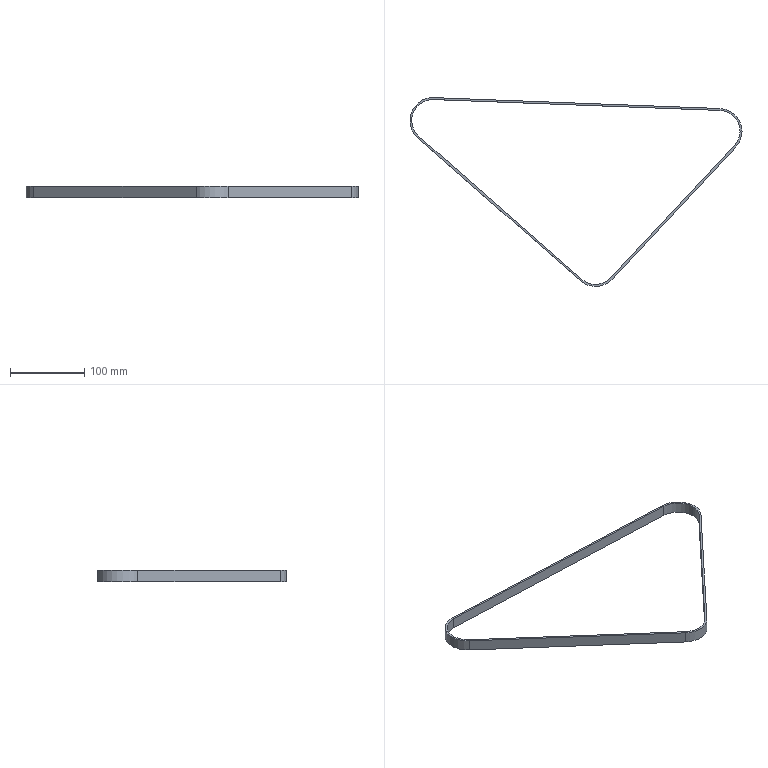Part | STEP file | Belt 2-5^ tube-changer assembly SGN-2 | 1 solid | 16 faces | box 446.051 x 253.563 x 15 mm | volume 43377 mm3 | cylinder 8 | plane 8 | commonest cylinder face diameters 56.34 x4 61.58 x4
STEP:
#1=CARTESIAN_POINT('',(0.,0.,0.));
#2=DIRECTION('',(0.,0.,1.));
#3=DIRECTION('',(1.,0.,0.));
#4=AXIS2_PLACEMENT_3D('',#1,#2,#3);
#5=CARTESIAN_POINT('',(-24.996,40.281,-15.));
#6=VERTEX_POINT('',#5);
#7=CARTESIAN_POINT('',(-24.996,40.281,0.));
#8=VERTEX_POINT('',#7);
#9=CARTESIAN_POINT('',(-24.996,40.281,-15.));
#10=DIRECTION('',(0.,0.,1.));
#11=VECTOR('',#10,1.);
#12=LINE('',#9,#11);
#13=CARTESIAN_POINT('',(-26.065,12.131,-15.));
#14=DIRECTION('',(0.,0.,1.));
#15=DIRECTION('',(1.,0.,0.));
#16=AXIS2_PLACEMENT_3D('',#13,#14,#15);
#17=CYLINDRICAL_SURFACE('',#16,28.17);
#18=CARTESIAN_POINT('',(1.533,0.));
#19=DIRECTION('',(0.,1.));
#20=VECTOR('',#19,1.);
#21=LINE('',#18,#20);
#22=(GEOMETRIC_REPRESENTATION_CONTEXT(2)PARAMETRIC_REPRESENTATION_CONTEXT()REPRESENTATION_CONTEXT('',''));
#23=DEFINITIONAL_REPRESENTATION('',(#21),#22);
#24=PCURVE('',#17,#23);
#25=CARTESIAN_POINT('',(-24.996,40.281,-15.));
#26=DIRECTION('',(0.03795,0.9993,0.));
#27=DIRECTION('',(-0.9993,0.03795,0.));
#28=AXIS2_PLACEMENT_3D('',#25,#26,#27);
#29=PLANE('',#28);
#30=CARTESIAN_POINT('',(0.,0.));
#31=DIRECTION('',(0.,1.));
#32=VECTOR('',#31,1.);
#33=LINE('',#30,#32);
#34=(GEOMETRIC_REPRESENTATION_CONTEXT(2)PARAMETRIC_REPRESENTATION_CONTEXT()REPRESENTATION_CONTEXT('',''));
#35=DEFINITIONAL_REPRESENTATION('',(#33),#34);
#36=PCURVE('',#29,#35);
#37=SURFACE_CURVE('',#12,(#24,#36),.PCURVE_S1.);
#38=EDGE_CURVE('',#6,#8,#37,.T.);
#39=ORIENTED_EDGE('',*,*,#38,.T.);
#40=CARTESIAN_POINT('',(2.105,12.131,0.));
#41=VERTEX_POINT('',#40);
#42=CARTESIAN_POINT('',(-26.065,12.131,0.));
#43=DIRECTION('',(0.,0.,1.));
#44=DIRECTION('',(1.,0.,0.));
#45=AXIS2_PLACEMENT_3D('',#42,#43,#44);
#46=CIRCLE('',#45,28.17);
#47=CARTESIAN_POINT('',(0.,15.));
#48=DIRECTION('',(1.,0.));
#49=VECTOR('',#48,1.);
#50=LINE('',#47,#49);
#51=(GEOMETRIC_REPRESENTATION_CONTEXT(2)PARAMETRIC_REPRESENTATION_CONTEXT()REPRESENTATION_CONTEXT('',''));
#52=DEFINITIONAL_REPRESENTATION('',(#50),#51);
#53=PCURVE('',#17,#52);
#54=CARTESIAN_POINT('',(-26.065,12.131,0.));
#55=DIRECTION('',(0.,0.,1.));
#56=DIRECTION('',(1.,0.,0.));
#57=AXIS2_PLACEMENT_3D('',#54,#55,#56);
#58=PLANE('',#57);
#59=CARTESIAN_POINT('',(0.,0.));
#60=DIRECTION('',(1.,0.));
#61=AXIS2_PLACEMENT_2D('',#59,#60);
#62=CIRCLE('',#61,28.17);
#63=(GEOMETRIC_REPRESENTATION_CONTEXT(2)PARAMETRIC_REPRESENTATION_CONTEXT()REPRESENTATION_CONTEXT('',''));
#64=DEFINITIONAL_REPRESENTATION('',(#62),#63);
#65=PCURVE('',#58,#64);
#66=SURFACE_CURVE('',#46,(#53,#65),.PCURVE_S1.);
#67=EDGE_CURVE('',#41,#8,#66,.T.);
#68=ORIENTED_EDGE('',*,*,#67,.F.);
#69=CARTESIAN_POINT('',(2.105,12.131,-15.));
#70=VERTEX_POINT('',#69);
#71=CARTESIAN_POINT('',(2.105,12.131,-15.));
#72=DIRECTION('',(0.,0.,1.));
#73=VECTOR('',#72,1.);
#74=LINE('',#71,#73);
#75=CARTESIAN_POINT('',(0.,0.));
#76=DIRECTION('',(0.,1.));
#77=VECTOR('',#76,1.);
#78=LINE('',#75,#77);
#79=(GEOMETRIC_REPRESENTATION_CONTEXT(2)PARAMETRIC_REPRESENTATION_CONTEXT()REPRESENTATION_CONTEXT('',''));
#80=DEFINITIONAL_REPRESENTATION('',(#78),#79);
#81=PCURVE('',#17,#80);
#82=CARTESIAN_POINT('',(-26.065,12.131,-15.));
#83=DIRECTION('',(0.,0.,1.));
#84=DIRECTION('',(1.,0.,0.));
#85=AXIS2_PLACEMENT_3D('',#82,#83,#84);
#86=CYLINDRICAL_SURFACE('',#85,28.17);
#87=CARTESIAN_POINT('',(6.283,0.));
#88=DIRECTION('',(0.,1.));
#89=VECTOR('',#88,1.);
#90=LINE('',#87,#89);
#91=(GEOMETRIC_REPRESENTATION_CONTEXT(2)PARAMETRIC_REPRESENTATION_CONTEXT()REPRESENTATION_CONTEXT('',''));
#92=DEFINITIONAL_REPRESENTATION('',(#90),#91);
#93=PCURVE('',#86,#92);
#94=SURFACE_CURVE('',#74,(#81,#93),.PCURVE_S1.);
#95=EDGE_CURVE('',#70,#41,#94,.T.);
#96=ORIENTED_EDGE('',*,*,#95,.F.);
#97=CARTESIAN_POINT('',(-26.065,12.131,-15.));
#98=DIRECTION('',(0.,0.,1.));
#99=DIRECTION('',(1.,0.,0.));
#100=AXIS2_PLACEMENT_3D('',#97,#98,#99);
#101=CIRCLE('',#100,28.17);
#102=CARTESIAN_POINT('',(0.,0.));
#103=DIRECTION('',(1.,0.));
#104=VECTOR('',#103,1.);
#105=LINE('',#102,#104);
#106=(GEOMETRIC_REPRESENTATION_CONTEXT(2)PARAMETRIC_REPRESENTATION_CONTEXT()REPRESENTATION_CONTEXT('',''));
#107=DEFINITIONAL_REPRESENTATION('',(#105),#106);
#108=PCURVE('',#17,#107);
#109=CARTESIAN_POINT('',(-26.065,12.131,-15.));
#110=DIRECTION('',(0.,0.,1.));
#111=DIRECTION('',(1.,0.,0.));
#112=AXIS2_PLACEMENT_3D('',#109,#110,#111);
#113=PLANE('',#112);
#114=CARTESIAN_POINT('',(0.,0.));
#115=DIRECTION('',(1.,0.));
#116=AXIS2_PLACEMENT_2D('',#114,#115);
#117=CIRCLE('',#116,28.17);
#118=(GEOMETRIC_REPRESENTATION_CONTEXT(2)PARAMETRIC_REPRESENTATION_CONTEXT()REPRESENTATION_CONTEXT('',''));
#119=DEFINITIONAL_REPRESENTATION('',(#117),#118);
#120=PCURVE('',#113,#119);
#121=SURFACE_CURVE('',#101,(#108,#120),.PCURVE_S1.);
#122=EDGE_CURVE('',#70,#6,#121,.T.);
#123=ORIENTED_EDGE('',*,*,#122,.T.);
#124=EDGE_LOOP('',(#39,#68,#96,#123));
#125=FACE_BOUND('',#124,.F.);
#126=ADVANCED_FACE('',(#125),#17,.F.);
#127=CARTESIAN_POINT('',(-3.587,-8.911,-15.));
#128=VERTEX_POINT('',#127);
#129=CARTESIAN_POINT('',(4.725,12.131,-15.));
#130=VERTEX_POINT('',#129);
#131=CARTESIAN_POINT('',(-26.065,12.131,-15.));
#132=DIRECTION('',(0.,0.,1.));
#133=DIRECTION('',(1.,0.,0.));
#134=AXIS2_PLACEMENT_3D('',#131,#132,#133);
#135=CIRCLE('',#134,30.79);
#136=CARTESIAN_POINT('',(-26.065,12.131,-15.));
#137=DIRECTION('',(0.,0.,1.));
#138=DIRECTION('',(1.,0.,0.));
#139=AXIS2_PLACEMENT_3D('',#136,#137,#138);
#140=CYLINDRICAL_SURFACE('',#139,30.79);
#141=CARTESIAN_POINT('',(0.,0.));
#142=DIRECTION('',(1.,0.));
#143=VECTOR('',#142,1.);
#144=LINE('',#141,#143);
#145=(GEOMETRIC_REPRESENTATION_CONTEXT(2)PARAMETRIC_REPRESENTATION_CONTEXT()REPRESENTATION_CONTEXT('',''));
#146=DEFINITIONAL_REPRESENTATION('',(#144),#145);
#147=PCURVE('',#140,#146);
#148=CARTESIAN_POINT('',(0.,0.));
#149=DIRECTION('',(1.,0.));
#150=AXIS2_PLACEMENT_2D('',#148,#149);
#151=CIRCLE('',#150,30.79);
#152=(GEOMETRIC_REPRESENTATION_CONTEXT(2)PARAMETRIC_REPRESENTATION_CONTEXT()REPRESENTATION_CONTEXT('',''));
#153=DEFINITIONAL_REPRESENTATION('',(#151),#152);
#154=PCURVE('',#113,#153);
#155=SURFACE_CURVE('',#135,(#147,#154),.PCURVE_S1.);
#156=EDGE_CURVE('',#128,#130,#155,.T.);
#157=ORIENTED_EDGE('',*,*,#156,.T.);
#158=CARTESIAN_POINT('',(4.725,12.131,0.));
#159=VERTEX_POINT('',#158);
#160=CARTESIAN_POINT('',(4.725,12.131,-15.));
#161=DIRECTION('',(0.,0.,1.));
#162=VECTOR('',#161,1.);
#163=LINE('',#160,#162);
#164=CARTESIAN_POINT('',(6.283,0.));
#165=DIRECTION('',(0.,1.));
#166=VECTOR('',#165,1.);
#167=LINE('',#164,#166);
#168=(GEOMETRIC_REPRESENTATION_CONTEXT(2)PARAMETRIC_REPRESENTATION_CONTEXT()REPRESENTATION_CONTEXT('',''));
#169=DEFINITIONAL_REPRESENTATION('',(#167),#168);
#170=PCURVE('',#140,#169);
#171=CARTESIAN_POINT('',(-26.065,12.131,-15.));
#172=DIRECTION('',(0.,0.,1.));
#173=DIRECTION('',(1.,0.,0.));
#174=AXIS2_PLACEMENT_3D('',#171,#172,#173);
#175=CYLINDRICAL_SURFACE('',#174,30.79);
#176=CARTESIAN_POINT('',(0.,0.));
#177=DIRECTION('',(0.,1.));
#178=VECTOR('',#177,1.);
#179=LINE('',#176,#178);
#180=(GEOMETRIC_REPRESENTATION_CONTEXT(2)PARAMETRIC_REPRESENTATION_CONTEXT()REPRESENTATION_CONTEXT('',''));
#181=DEFINITIONAL_REPRESENTATION('',(#179),#180);
#182=PCURVE('',#175,#181);
#183=SURFACE_CURVE('',#163,(#170,#182),.PCURVE_S1.);
#184=EDGE_CURVE('',#130,#159,#183,.T.);
#185=ORIENTED_EDGE('',*,*,#184,.T.);
#186=CARTESIAN_POINT('',(-3.587,-8.911,0.));
#187=VERTEX_POINT('',#186);
#188=CARTESIAN_POINT('',(-26.065,12.131,0.));
#189=DIRECTION('',(0.,0.,1.));
#190=DIRECTION('',(1.,0.,0.));
#191=AXIS2_PLACEMENT_3D('',#188,#189,#190);
#192=CIRCLE('',#191,30.79);
#193=CARTESIAN_POINT('',(0.,15.));
#194=DIRECTION('',(1.,0.));
#195=VECTOR('',#194,1.);
#196=LINE('',#193,#195);
#197=(GEOMETRIC_REPRESENTATION_CONTEXT(2)PARAMETRIC_REPRESENTATION_CONTEXT()REPRESENTATION_CONTEXT('',''));
#198=DEFINITIONAL_REPRESENTATION('',(#196),#197);
#199=PCURVE('',#140,#198);
#200=CARTESIAN_POINT('',(0.,0.));
#201=DIRECTION('',(1.,0.));
#202=AXIS2_PLACEMENT_2D('',#200,#201);
#203=CIRCLE('',#202,30.79);
#204=(GEOMETRIC_REPRESENTATION_CONTEXT(2)PARAMETRIC_REPRESENTATION_CONTEXT()REPRESENTATION_CONTEXT('',''));
#205=DEFINITIONAL_REPRESENTATION('',(#203),#204);
#206=PCURVE('',#58,#205);
#207=SURFACE_CURVE('',#192,(#199,#206),.PCURVE_S1.);
#208=EDGE_CURVE('',#187,#159,#207,.T.);
#209=ORIENTED_EDGE('',*,*,#208,.F.);
#210=CARTESIAN_POINT('',(-3.587,-8.911,-15.));
#211=DIRECTION('',(0.,0.,1.));
#212=VECTOR('',#211,1.);
#213=LINE('',#210,#212);
#214=CARTESIAN_POINT('',(5.531,0.));
#215=DIRECTION('',(0.,1.));
#216=VECTOR('',#215,1.);
#217=LINE('',#214,#216);
#218=(GEOMETRIC_REPRESENTATION_CONTEXT(2)PARAMETRIC_REPRESENTATION_CONTEXT()REPRESENTATION_CONTEXT('',''));
#219=DEFINITIONAL_REPRESENTATION('',(#217),#218);
#220=PCURVE('',#140,#219);
#221=CARTESIAN_POINT('',(-169.638,-186.293,-15.));
#222=DIRECTION('',(0.73,-0.6834,0.));
#223=DIRECTION('',(0.6834,0.73,0.));
#224=AXIS2_PLACEMENT_3D('',#221,#222,#223);
#225=PLANE('',#224);
#226=CARTESIAN_POINT('',(242.976,0.));
#227=DIRECTION('',(0.,1.));
#228=VECTOR('',#227,1.);
#229=LINE('',#226,#228);
#230=(GEOMETRIC_REPRESENTATION_CONTEXT(2)PARAMETRIC_REPRESENTATION_CONTEXT()REPRESENTATION_CONTEXT('',''));
#231=DEFINITIONAL_REPRESENTATION('',(#229),#230);
#232=PCURVE('',#225,#231);
#233=SURFACE_CURVE('',#213,(#220,#232),.PCURVE_S1.);
#234=EDGE_CURVE('',#128,#187,#233,.T.);
#235=ORIENTED_EDGE('',*,*,#234,.F.);
#236=EDGE_LOOP('',(#157,#185,#209,#235));
#237=FACE_BOUND('',#236,.T.);
#238=ADVANCED_FACE('',(#237),#140,.T.);
#239=ORIENTED_EDGE('',*,*,#184,.F.);
#240=CARTESIAN_POINT('',(-24.897,42.899,-15.));
#241=VERTEX_POINT('',#240);
#242=CARTESIAN_POINT('',(-26.065,12.131,-15.));
#243=DIRECTION('',(0.,0.,1.));
#244=DIRECTION('',(1.,0.,0.));
#245=AXIS2_PLACEMENT_3D('',#242,#243,#244);
#246=CIRCLE('',#245,30.79);
#247=CARTESIAN_POINT('',(0.,0.));
#248=DIRECTION('',(1.,0.));
#249=VECTOR('',#248,1.);
#250=LINE('',#247,#249);
#251=(GEOMETRIC_REPRESENTATION_CONTEXT(2)PARAMETRIC_REPRESENTATION_CONTEXT()REPRESENTATION_CONTEXT('',''));
#252=DEFINITIONAL_REPRESENTATION('',(#250),#251);
#253=PCURVE('',#175,#252);
#254=CARTESIAN_POINT('',(0.,0.));
#255=DIRECTION('',(1.,0.));
#256=AXIS2_PLACEMENT_2D('',#254,#255);
#257=CIRCLE('',#256,30.79);
#258=(GEOMETRIC_REPRESENTATION_CONTEXT(2)PARAMETRIC_REPRESENTATION_CONTEXT()REPRESENTATION_CONTEXT('',''));
#259=DEFINITIONAL_REPRESENTATION('',(#257),#258);
#260=PCURVE('',#113,#259);
#261=SURFACE_CURVE('',#246,(#253,#260),.PCURVE_S1.);
#262=EDGE_CURVE('',#130,#241,#261,.T.);
#263=ORIENTED_EDGE('',*,*,#262,.T.);
#264=CARTESIAN_POINT('',(-24.897,42.899,0.));
#265=VERTEX_POINT('',#264);
#266=CARTESIAN_POINT('',(-24.897,42.899,-15.));
#267=DIRECTION('',(0.,0.,1.));
#268=VECTOR('',#267,1.);
#269=LINE('',#266,#268);
#270=CARTESIAN_POINT('',(1.533,0.));
#271=DIRECTION('',(0.,1.));
#272=VECTOR('',#271,1.);
#273=LINE('',#270,#272);
#274=(GEOMETRIC_REPRESENTATION_CONTEXT(2)PARAMETRIC_REPRESENTATION_CONTEXT()REPRESENTATION_CONTEXT('',''));
#275=DEFINITIONAL_REPRESENTATION('',(#273),#274);
#276=PCURVE('',#175,#275);
#277=CARTESIAN_POINT('',(-24.897,42.899,-15.));
#278=DIRECTION('',(0.03795,0.9993,0.));
#279=DIRECTION('',(-0.9993,0.03795,0.));
#280=AXIS2_PLACEMENT_3D('',#277,#278,#279);
#281=PLANE('',#280);
#282=CARTESIAN_POINT('',(0.,0.));
#283=DIRECTION('',(0.,1.));
#284=VECTOR('',#283,1.);
#285=LINE('',#282,#284);
#286=(GEOMETRIC_REPRESENTATION_CONTEXT(2)PARAMETRIC_REPRESENTATION_CONTEXT()REPRESENTATION_CONTEXT('',''));
#287=DEFINITIONAL_REPRESENTATION('',(#285),#286);
#288=PCURVE('',#281,#287);
#289=SURFACE_CURVE('',#269,(#276,#288),.PCURVE_S1.);
#290=EDGE_CURVE('',#241,#265,#289,.T.);
#291=ORIENTED_EDGE('',*,*,#290,.T.);
#292=CARTESIAN_POINT('',(-26.065,12.131,0.));
#293=DIRECTION('',(0.,0.,1.));
#294=DIRECTION('',(1.,0.,0.));
#295=AXIS2_PLACEMENT_3D('',#292,#293,#294);
#296=CIRCLE('',#295,30.79);
#297=CARTESIAN_POINT('',(0.,15.));
#298=DIRECTION('',(1.,0.));
#299=VECTOR('',#298,1.);
#300=LINE('',#297,#299);
#301=(GEOMETRIC_REPRESENTATION_CONTEXT(2)PARAMETRIC_REPRESENTATION_CONTEXT()REPRESENTATION_CONTEXT('',''));
#302=DEFINITIONAL_REPRESENTATION('',(#300),#301);
#303=PCURVE('',#175,#302);
#304=CARTESIAN_POINT('',(0.,0.));
#305=DIRECTION('',(1.,0.));
#306=AXIS2_PLACEMENT_2D('',#304,#305);
#307=CIRCLE('',#306,30.79);
#308=(GEOMETRIC_REPRESENTATION_CONTEXT(2)PARAMETRIC_REPRESENTATION_CONTEXT()REPRESENTATION_CONTEXT('',''));
#309=DEFINITIONAL_REPRESENTATION('',(#307),#308);
#310=PCURVE('',#58,#309);
#311=SURFACE_CURVE('',#296,(#303,#310),.PCURVE_S1.);
#312=EDGE_CURVE('',#159,#265,#311,.T.);
#313=ORIENTED_EDGE('',*,*,#312,.F.);
#314=EDGE_LOOP('',(#239,#263,#291,#313));
#315=FACE_BOUND('',#314,.T.);
#316=ADVANCED_FACE('',(#315),#175,.T.);
#317=CARTESIAN_POINT('',(-169.638,-186.293,0.));
#318=VERTEX_POINT('',#317);
#319=CARTESIAN_POINT('',(-169.638,-186.293,0.));
#320=DIRECTION('',(0.6834,0.73,0.));
#321=VECTOR('',#320,1.);
#322=LINE('',#319,#321);
#323=CARTESIAN_POINT('',(0.,15.));
#324=DIRECTION('',(1.,0.));
#325=VECTOR('',#324,1.);
#326=LINE('',#323,#325);
#327=(GEOMETRIC_REPRESENTATION_CONTEXT(2)PARAMETRIC_REPRESENTATION_CONTEXT()REPRESENTATION_CONTEXT('',''));
#328=DEFINITIONAL_REPRESENTATION('',(#326),#327);
#329=PCURVE('',#225,#328);
#330=CARTESIAN_POINT('',(-143.572,-198.424));
#331=DIRECTION('',(0.6834,0.73));
#332=VECTOR('',#331,1.);
#333=LINE('',#330,#332);
#334=(GEOMETRIC_REPRESENTATION_CONTEXT(2)PARAMETRIC_REPRESENTATION_CONTEXT()REPRESENTATION_CONTEXT('',''));
#335=DEFINITIONAL_REPRESENTATION('',(#333),#334);
#336=PCURVE('',#58,#335);
#337=SURFACE_CURVE('',#322,(#329,#336),.PCURVE_S1.);
#338=EDGE_CURVE('',#318,#187,#337,.T.);
#339=ORIENTED_EDGE('',*,*,#338,.F.);
#340=CARTESIAN_POINT('',(-169.638,-186.293,-15.));
#341=VERTEX_POINT('',#340);
#342=CARTESIAN_POINT('',(-169.638,-186.293,-15.));
#343=DIRECTION('',(0.,0.,1.));
#344=VECTOR('',#343,1.);
#345=LINE('',#342,#344);
#346=CARTESIAN_POINT('',(0.,0.));
#347=DIRECTION('',(0.,1.));
#348=VECTOR('',#347,1.);
#349=LINE('',#346,#348);
#350=(GEOMETRIC_REPRESENTATION_CONTEXT(2)PARAMETRIC_REPRESENTATION_CONTEXT()REPRESENTATION_CONTEXT('',''));
#351=DEFINITIONAL_REPRESENTATION('',(#349),#350);
#352=PCURVE('',#225,#351);
#353=CARTESIAN_POINT('',(-192.116,-165.251,-15.));
#354=DIRECTION('',(0.,0.,1.));
#355=DIRECTION('',(1.,0.,0.));
#356=AXIS2_PLACEMENT_3D('',#353,#354,#355);
#357=CYLINDRICAL_SURFACE('',#356,30.79);
#358=CARTESIAN_POINT('',(5.531,0.));
#359=DIRECTION('',(0.,1.));
#360=VECTOR('',#359,1.);
#361=LINE('',#358,#360);
#362=(GEOMETRIC_REPRESENTATION_CONTEXT(2)PARAMETRIC_REPRESENTATION_CONTEXT()REPRESENTATION_CONTEXT('',''));
#363=DEFINITIONAL_REPRESENTATION('',(#361),#362);
#364=PCURVE('',#357,#363);
#365=SURFACE_CURVE('',#345,(#352,#364),.PCURVE_S1.);
#366=EDGE_CURVE('',#341,#318,#365,.T.);
#367=ORIENTED_EDGE('',*,*,#366,.F.);
#368=CARTESIAN_POINT('',(-169.638,-186.293,-15.));
#369=DIRECTION('',(0.6834,0.73,0.));
#370=VECTOR('',#369,1.);
#371=LINE('',#368,#370);
#372=CARTESIAN_POINT('',(0.,0.));
#373=DIRECTION('',(1.,0.));
#374=VECTOR('',#373,1.);
#375=LINE('',#372,#374);
#376=(GEOMETRIC_REPRESENTATION_CONTEXT(2)PARAMETRIC_REPRESENTATION_CONTEXT()REPRESENTATION_CONTEXT('',''));
#377=DEFINITIONAL_REPRESENTATION('',(#375),#376);
#378=PCURVE('',#225,#377);
#379=CARTESIAN_POINT('',(-143.572,-198.424));
#380=DIRECTION('',(0.6834,0.73));
#381=VECTOR('',#380,1.);
#382=LINE('',#379,#381);
#383=(GEOMETRIC_REPRESENTATION_CONTEXT(2)PARAMETRIC_REPRESENTATION_CONTEXT()REPRESENTATION_CONTEXT('',''));
#384=DEFINITIONAL_REPRESENTATION('',(#382),#383);
#385=PCURVE('',#113,#384);
#386=SURFACE_CURVE('',#371,(#378,#385),.PCURVE_S1.);
#387=EDGE_CURVE('',#341,#128,#386,.T.);
#388=ORIENTED_EDGE('',*,*,#387,.T.);
#389=ORIENTED_EDGE('',*,*,#234,.T.);
#390=EDGE_LOOP('',(#339,#367,#388,#389));
#391=FACE_BOUND('',#390,.T.);
#392=ADVANCED_FACE('',(#391),#225,.T.);
#393=CARTESIAN_POINT('',(-212.443,-188.378,0.));
#394=VERTEX_POINT('',#393);
#395=CARTESIAN_POINT('',(-192.116,-165.251,0.));
#396=DIRECTION('',(0.,0.,1.));
#397=DIRECTION('',(1.,0.,0.));
#398=AXIS2_PLACEMENT_3D('',#395,#396,#397);
#399=CIRCLE('',#398,30.79);
#400=CARTESIAN_POINT('',(0.,15.));
#401=DIRECTION('',(1.,0.));
#402=VECTOR('',#401,1.);
#403=LINE('',#400,#402);
#404=(GEOMETRIC_REPRESENTATION_CONTEXT(2)PARAMETRIC_REPRESENTATION_CONTEXT()REPRESENTATION_CONTEXT('',''));
#405=DEFINITIONAL_REPRESENTATION('',(#403),#404);
#406=PCURVE('',#357,#405);
#407=CARTESIAN_POINT('',(-166.05,-177.382));
#408=DIRECTION('',(1.,0.));
#409=AXIS2_PLACEMENT_2D('',#407,#408);
#410=CIRCLE('',#409,30.79);
#411=(GEOMETRIC_REPRESENTATION_CONTEXT(2)PARAMETRIC_REPRESENTATION_CONTEXT()REPRESENTATION_CONTEXT('',''));
#412=DEFINITIONAL_REPRESENTATION('',(#410),#411);
#413=PCURVE('',#58,#412);
#414=SURFACE_CURVE('',#399,(#406,#413),.PCURVE_S1.);
#415=EDGE_CURVE('',#394,#318,#414,.T.);
#416=ORIENTED_EDGE('',*,*,#415,.F.);
#417=CARTESIAN_POINT('',(-212.443,-188.378,-15.));
#418=VERTEX_POINT('',#417);
#419=CARTESIAN_POINT('',(-212.443,-188.378,-15.));
#420=DIRECTION('',(0.,0.,1.));
#421=VECTOR('',#420,1.);
#422=LINE('',#419,#421);
#423=CARTESIAN_POINT('',(3.991,0.));
#424=DIRECTION('',(0.,1.));
#425=VECTOR('',#424,1.);
#426=LINE('',#423,#425);
#427=(GEOMETRIC_REPRESENTATION_CONTEXT(2)PARAMETRIC_REPRESENTATION_CONTEXT()REPRESENTATION_CONTEXT('',''));
#428=DEFINITIONAL_REPRESENTATION('',(#426),#427);
#429=PCURVE('',#357,#428);
#430=CARTESIAN_POINT('',(-430.863,3.605,-15.));
#431=DIRECTION('',(-0.6602,-0.7511,0.));
#432=DIRECTION('',(0.7511,-0.6602,0.));
#433=AXIS2_PLACEMENT_3D('',#430,#431,#432);
#434=PLANE('',#433);
#435=CARTESIAN_POINT('',(290.8,0.));
#436=DIRECTION('',(0.,1.));
#437=VECTOR('',#436,1.);
#438=LINE('',#435,#437);
#439=(GEOMETRIC_REPRESENTATION_CONTEXT(2)PARAMETRIC_REPRESENTATION_CONTEXT()REPRESENTATION_CONTEXT('',''));
#440=DEFINITIONAL_REPRESENTATION('',(#438),#439);
#441=PCURVE('',#434,#440);
#442=SURFACE_CURVE('',#422,(#429,#441),.PCURVE_S1.);
#443=EDGE_CURVE('',#418,#394,#442,.T.);
#444=ORIENTED_EDGE('',*,*,#443,.F.);
#445=CARTESIAN_POINT('',(-192.116,-165.251,-15.));
#446=DIRECTION('',(0.,0.,1.));
#447=DIRECTION('',(1.,0.,0.));
#448=AXIS2_PLACEMENT_3D('',#445,#446,#447);
#449=CIRCLE('',#448,30.79);
#450=CARTESIAN_POINT('',(0.,0.));
#451=DIRECTION('',(1.,0.));
#452=VECTOR('',#451,1.);
#453=LINE('',#450,#452);
#454=(GEOMETRIC_REPRESENTATION_CONTEXT(2)PARAMETRIC_REPRESENTATION_CONTEXT()REPRESENTATION_CONTEXT('',''));
#455=DEFINITIONAL_REPRESENTATION('',(#453),#454);
#456=PCURVE('',#357,#455);
#457=CARTESIAN_POINT('',(-166.05,-177.382));
#458=DIRECTION('',(1.,0.));
#459=AXIS2_PLACEMENT_2D('',#457,#458);
#460=CIRCLE('',#459,30.79);
#461=(GEOMETRIC_REPRESENTATION_CONTEXT(2)PARAMETRIC_REPRESENTATION_CONTEXT()REPRESENTATION_CONTEXT('',''));
#462=DEFINITIONAL_REPRESENTATION('',(#460),#461);
#463=PCURVE('',#113,#462);
#464=SURFACE_CURVE('',#449,(#456,#463),.PCURVE_S1.);
#465=EDGE_CURVE('',#418,#341,#464,.T.);
#466=ORIENTED_EDGE('',*,*,#465,.T.);
#467=ORIENTED_EDGE('',*,*,#366,.T.);
#468=EDGE_LOOP('',(#416,#444,#466,#467));
#469=FACE_BOUND('',#468,.T.);
#470=ADVANCED_FACE('',(#469),#357,.T.);
#471=CARTESIAN_POINT('',(-430.863,3.605,0.));
#472=VERTEX_POINT('',#471);
#473=CARTESIAN_POINT('',(-430.863,3.605,0.));
#474=DIRECTION('',(0.7511,-0.6602,0.));
#475=VECTOR('',#474,1.);
#476=LINE('',#473,#475);
#477=CARTESIAN_POINT('',(0.,15.));
#478=DIRECTION('',(1.,0.));
#479=VECTOR('',#478,1.);
#480=LINE('',#477,#479);
#481=(GEOMETRIC_REPRESENTATION_CONTEXT(2)PARAMETRIC_REPRESENTATION_CONTEXT()REPRESENTATION_CONTEXT('',''));
#482=DEFINITIONAL_REPRESENTATION('',(#480),#481);
#483=PCURVE('',#434,#482);
#484=CARTESIAN_POINT('',(-404.798,-8.526));
#485=DIRECTION('',(0.7511,-0.6602));
#486=VECTOR('',#485,1.);
#487=LINE('',#484,#486);
#488=(GEOMETRIC_REPRESENTATION_CONTEXT(2)PARAMETRIC_REPRESENTATION_CONTEXT()REPRESENTATION_CONTEXT('',''));
#489=DEFINITIONAL_REPRESENTATION('',(#487),#488);
#490=PCURVE('',#58,#489);
#491=SURFACE_CURVE('',#476,(#483,#490),.PCURVE_S1.);
#492=EDGE_CURVE('',#472,#394,#491,.T.);
#493=ORIENTED_EDGE('',*,*,#492,.F.);
#494=CARTESIAN_POINT('',(-430.863,3.605,-15.));
#495=VERTEX_POINT('',#494);
#496=CARTESIAN_POINT('',(-430.863,3.605,-15.));
#497=DIRECTION('',(0.,0.,1.));
#498=VECTOR('',#497,1.);
#499=LINE('',#496,#498);
#500=CARTESIAN_POINT('',(0.,0.));
#501=DIRECTION('',(0.,1.));
#502=VECTOR('',#501,1.);
#503=LINE('',#500,#502);
#504=(GEOMETRIC_REPRESENTATION_CONTEXT(2)PARAMETRIC_REPRESENTATION_CONTEXT()REPRESENTATION_CONTEXT('',''));
#505=DEFINITIONAL_REPRESENTATION('',(#503),#504);
#506=PCURVE('',#434,#505);
#507=CARTESIAN_POINT('',(-410.536,26.731,-15.));
#508=DIRECTION('',(0.,0.,1.));
#509=DIRECTION('',(1.,0.,0.));
#510=AXIS2_PLACEMENT_3D('',#507,#508,#509);
#511=CYLINDRICAL_SURFACE('',#510,30.79);
#512=CARTESIAN_POINT('',(3.991,0.));
#513=DIRECTION('',(0.,1.));
#514=VECTOR('',#513,1.);
#515=LINE('',#512,#514);
#516=(GEOMETRIC_REPRESENTATION_CONTEXT(2)PARAMETRIC_REPRESENTATION_CONTEXT()REPRESENTATION_CONTEXT('',''));
#517=DEFINITIONAL_REPRESENTATION('',(#515),#516);
#518=PCURVE('',#511,#517);
#519=SURFACE_CURVE('',#499,(#506,#518),.PCURVE_S1.);
#520=EDGE_CURVE('',#495,#472,#519,.T.);
#521=ORIENTED_EDGE('',*,*,#520,.F.);
#522=CARTESIAN_POINT('',(-430.863,3.605,-15.));
#523=DIRECTION('',(0.7511,-0.6602,0.));
#524=VECTOR('',#523,1.);
#525=LINE('',#522,#524);
#526=CARTESIAN_POINT('',(0.,0.));
#527=DIRECTION('',(1.,0.));
#528=VECTOR('',#527,1.);
#529=LINE('',#526,#528);
#530=(GEOMETRIC_REPRESENTATION_CONTEXT(2)PARAMETRIC_REPRESENTATION_CONTEXT()REPRESENTATION_CONTEXT('',''));
#531=DEFINITIONAL_REPRESENTATION('',(#529),#530);
#532=PCURVE('',#434,#531);
#533=CARTESIAN_POINT('',(-404.798,-8.526));
#534=DIRECTION('',(0.7511,-0.6602));
#535=VECTOR('',#534,1.);
#536=LINE('',#533,#535);
#537=(GEOMETRIC_REPRESENTATION_CONTEXT(2)PARAMETRIC_REPRESENTATION_CONTEXT()REPRESENTATION_CONTEXT('',''));
#538=DEFINITIONAL_REPRESENTATION('',(#536),#537);
#539=PCURVE('',#113,#538);
#540=SURFACE_CURVE('',#525,(#532,#539),.PCURVE_S1.);
#541=EDGE_CURVE('',#495,#418,#540,.T.);
#542=ORIENTED_EDGE('',*,*,#541,.T.);
#543=ORIENTED_EDGE('',*,*,#443,.T.);
#544=EDGE_LOOP('',(#493,#521,#542,#543));
#545=FACE_BOUND('',#544,.T.);
#546=ADVANCED_FACE('',(#545),#434,.T.);
#547=CARTESIAN_POINT('',(-409.368,57.499,0.));
#548=VERTEX_POINT('',#547);
#549=CARTESIAN_POINT('',(-410.536,26.731,0.));
#550=DIRECTION('',(0.,0.,1.));
#551=DIRECTION('',(1.,0.,0.));
#552=AXIS2_PLACEMENT_3D('',#549,#550,#551);
#553=CIRCLE('',#552,30.79);
#554=CARTESIAN_POINT('',(0.,15.));
#555=DIRECTION('',(1.,0.));
#556=VECTOR('',#555,1.);
#557=LINE('',#554,#556);
#558=(GEOMETRIC_REPRESENTATION_CONTEXT(2)PARAMETRIC_REPRESENTATION_CONTEXT()REPRESENTATION_CONTEXT('',''));
#559=DEFINITIONAL_REPRESENTATION('',(#557),#558);
#560=PCURVE('',#511,#559);
#561=CARTESIAN_POINT('',(-384.471,14.6));
#562=DIRECTION('',(1.,0.));
#563=AXIS2_PLACEMENT_2D('',#561,#562);
#564=CIRCLE('',#563,30.79);
#565=(GEOMETRIC_REPRESENTATION_CONTEXT(2)PARAMETRIC_REPRESENTATION_CONTEXT()REPRESENTATION_CONTEXT('',''));
#566=DEFINITIONAL_REPRESENTATION('',(#564),#565);
#567=PCURVE('',#58,#566);
#568=SURFACE_CURVE('',#553,(#560,#567),.PCURVE_S1.);
#569=EDGE_CURVE('',#548,#472,#568,.T.);
#570=ORIENTED_EDGE('',*,*,#569,.F.);
#571=CARTESIAN_POINT('',(-409.368,57.499,-15.));
#572=VERTEX_POINT('',#571);
#573=CARTESIAN_POINT('',(-409.368,57.499,-15.));
#574=DIRECTION('',(0.,0.,1.));
#575=VECTOR('',#574,1.);
#576=LINE('',#573,#575);
#577=CARTESIAN_POINT('',(1.533,0.));
#578=DIRECTION('',(0.,1.));
#579=VECTOR('',#578,1.);
#580=LINE('',#577,#579);
#581=(GEOMETRIC_REPRESENTATION_CONTEXT(2)PARAMETRIC_REPRESENTATION_CONTEXT()REPRESENTATION_CONTEXT('',''));
#582=DEFINITIONAL_REPRESENTATION('',(#580),#581);
#583=PCURVE('',#511,#582);
#584=CARTESIAN_POINT('',(384.748,0.));
#585=DIRECTION('',(0.,1.));
#586=VECTOR('',#585,1.);
#587=LINE('',#584,#586);
#588=(GEOMETRIC_REPRESENTATION_CONTEXT(2)PARAMETRIC_REPRESENTATION_CONTEXT()REPRESENTATION_CONTEXT('',''));
#589=DEFINITIONAL_REPRESENTATION('',(#587),#588);
#590=PCURVE('',#281,#589);
#591=SURFACE_CURVE('',#576,(#583,#590),.PCURVE_S1.);
#592=EDGE_CURVE('',#572,#548,#591,.T.);
#593=ORIENTED_EDGE('',*,*,#592,.F.);
#594=CARTESIAN_POINT('',(-410.536,26.731,-15.));
#595=DIRECTION('',(0.,0.,1.));
#596=DIRECTION('',(1.,0.,0.));
#597=AXIS2_PLACEMENT_3D('',#594,#595,#596);
#598=CIRCLE('',#597,30.79);
#599=CARTESIAN_POINT('',(0.,0.));
#600=DIRECTION('',(1.,0.));
#601=VECTOR('',#600,1.);
#602=LINE('',#599,#601);
#603=(GEOMETRIC_REPRESENTATION_CONTEXT(2)PARAMETRIC_REPRESENTATION_CONTEXT()REPRESENTATION_CONTEXT('',''));
#604=DEFINITIONAL_REPRESENTATION('',(#602),#603);
#605=PCURVE('',#511,#604);
#606=CARTESIAN_POINT('',(-384.471,14.6));
#607=DIRECTION('',(1.,0.));
#608=AXIS2_PLACEMENT_2D('',#606,#607);
#609=CIRCLE('',#608,30.79);
#610=(GEOMETRIC_REPRESENTATION_CONTEXT(2)PARAMETRIC_REPRESENTATION_CONTEXT()REPRESENTATION_CONTEXT('',''));
#611=DEFINITIONAL_REPRESENTATION('',(#609),#610);
#612=PCURVE('',#113,#611);
#613=SURFACE_CURVE('',#598,(#605,#612),.PCURVE_S1.);
#614=EDGE_CURVE('',#572,#495,#613,.T.);
#615=ORIENTED_EDGE('',*,*,#614,.T.);
#616=ORIENTED_EDGE('',*,*,#520,.T.);
#617=EDGE_LOOP('',(#570,#593,#615,#616));
#618=FACE_BOUND('',#617,.T.);
#619=ADVANCED_FACE('',(#618),#511,.T.);
#620=CARTESIAN_POINT('',(-24.897,42.899,0.));
#621=DIRECTION('',(-0.9993,0.03795,0.));
#622=VECTOR('',#621,1.);
#623=LINE('',#620,#622);
#624=CARTESIAN_POINT('',(0.,15.));
#625=DIRECTION('',(1.,0.));
#626=VECTOR('',#625,1.);
#627=LINE('',#624,#626);
#628=(GEOMETRIC_REPRESENTATION_CONTEXT(2)PARAMETRIC_REPRESENTATION_CONTEXT()REPRESENTATION_CONTEXT('',''));
#629=DEFINITIONAL_REPRESENTATION('',(#627),#628);
#630=PCURVE('',#281,#629);
#631=CARTESIAN_POINT('',(1.168,30.768));
#632=DIRECTION('',(-0.9993,0.03795));
#633=VECTOR('',#632,1.);
#634=LINE('',#631,#633);
#635=(GEOMETRIC_REPRESENTATION_CONTEXT(2)PARAMETRIC_REPRESENTATION_CONTEXT()REPRESENTATION_CONTEXT('',''));
#636=DEFINITIONAL_REPRESENTATION('',(#634),#635);
#637=PCURVE('',#58,#636);
#638=SURFACE_CURVE('',#623,(#630,#637),.PCURVE_S1.);
#639=EDGE_CURVE('',#265,#548,#638,.T.);
#640=ORIENTED_EDGE('',*,*,#639,.F.);
#641=ORIENTED_EDGE('',*,*,#290,.F.);
#642=CARTESIAN_POINT('',(-24.897,42.899,-15.));
#643=DIRECTION('',(-0.9993,0.03795,0.));
#644=VECTOR('',#643,1.);
#645=LINE('',#642,#644);
#646=CARTESIAN_POINT('',(0.,0.));
#647=DIRECTION('',(1.,0.));
#648=VECTOR('',#647,1.);
#649=LINE('',#646,#648);
#650=(GEOMETRIC_REPRESENTATION_CONTEXT(2)PARAMETRIC_REPRESENTATION_CONTEXT()REPRESENTATION_CONTEXT('',''));
#651=DEFINITIONAL_REPRESENTATION('',(#649),#650);
#652=PCURVE('',#281,#651);
#653=CARTESIAN_POINT('',(1.168,30.768));
#654=DIRECTION('',(-0.9993,0.03795));
#655=VECTOR('',#654,1.);
#656=LINE('',#653,#655);
#657=(GEOMETRIC_REPRESENTATION_CONTEXT(2)PARAMETRIC_REPRESENTATION_CONTEXT()REPRESENTATION_CONTEXT('',''));
#658=DEFINITIONAL_REPRESENTATION('',(#656),#657);
#659=PCURVE('',#113,#658);
#660=SURFACE_CURVE('',#645,(#652,#659),.PCURVE_S1.);
#661=EDGE_CURVE('',#241,#572,#660,.T.);
#662=ORIENTED_EDGE('',*,*,#661,.T.);
#663=ORIENTED_EDGE('',*,*,#592,.T.);
#664=EDGE_LOOP('',(#640,#641,#662,#663));
#665=FACE_BOUND('',#664,.T.);
#666=ADVANCED_FACE('',(#665),#281,.T.);
#667=CARTESIAN_POINT('',(-171.55,-184.503,-15.));
#668=VERTEX_POINT('',#667);
#669=CARTESIAN_POINT('',(-5.5,-7.12,-15.));
#670=VERTEX_POINT('',#669);
#671=CARTESIAN_POINT('',(-171.55,-184.503,-15.));
#672=DIRECTION('',(0.6834,0.73,0.));
#673=VECTOR('',#672,1.);
#674=LINE('',#671,#673);
#675=CARTESIAN_POINT('',(-145.485,-196.634));
#676=DIRECTION('',(0.6834,0.73));
#677=VECTOR('',#676,1.);
#678=LINE('',#675,#677);
#679=(GEOMETRIC_REPRESENTATION_CONTEXT(2)PARAMETRIC_REPRESENTATION_CONTEXT()REPRESENTATION_CONTEXT('',''));
#680=DEFINITIONAL_REPRESENTATION('',(#678),#679);
#681=PCURVE('',#113,#680);
#682=CARTESIAN_POINT('',(-171.55,-184.503,-15.));
#683=DIRECTION('',(0.73,-0.6834,0.));
#684=DIRECTION('',(0.6834,0.73,0.));
#685=AXIS2_PLACEMENT_3D('',#682,#683,#684);
#686=PLANE('',#685);
#687=CARTESIAN_POINT('',(0.,0.));
#688=DIRECTION('',(1.,0.));
#689=VECTOR('',#688,1.);
#690=LINE('',#687,#689);
#691=(GEOMETRIC_REPRESENTATION_CONTEXT(2)PARAMETRIC_REPRESENTATION_CONTEXT()REPRESENTATION_CONTEXT('',''));
#692=DEFINITIONAL_REPRESENTATION('',(#690),#691);
#693=PCURVE('',#686,#692);
#694=SURFACE_CURVE('',#674,(#681,#693),.PCURVE_S1.);
#695=EDGE_CURVE('',#668,#670,#694,.T.);
#696=ORIENTED_EDGE('',*,*,#695,.T.);
#697=CARTESIAN_POINT('',(-26.065,12.131,-15.));
#698=DIRECTION('',(0.,0.,1.));
#699=DIRECTION('',(1.,0.,0.));
#700=AXIS2_PLACEMENT_3D('',#697,#698,#699);
#701=CIRCLE('',#700,28.17);
#702=CARTESIAN_POINT('',(0.,0.));
#703=DIRECTION('',(1.,0.));
#704=AXIS2_PLACEMENT_2D('',#702,#703);
#705=CIRCLE('',#704,28.17);
#706=(GEOMETRIC_REPRESENTATION_CONTEXT(2)PARAMETRIC_REPRESENTATION_CONTEXT()REPRESENTATION_CONTEXT('',''));
#707=DEFINITIONAL_REPRESENTATION('',(#705),#706);
#708=PCURVE('',#113,#707);
#709=CARTESIAN_POINT('',(0.,0.));
#710=DIRECTION('',(1.,0.));
#711=VECTOR('',#710,1.);
#712=LINE('',#709,#711);
#713=(GEOMETRIC_REPRESENTATION_CONTEXT(2)PARAMETRIC_REPRESENTATION_CONTEXT()REPRESENTATION_CONTEXT('',''));
#714=DEFINITIONAL_REPRESENTATION('',(#712),#713);
#715=PCURVE('',#86,#714);
#716=SURFACE_CURVE('',#701,(#708,#715),.PCURVE_S1.);
#717=EDGE_CURVE('',#670,#70,#716,.T.);
#718=ORIENTED_EDGE('',*,*,#717,.T.);
#719=ORIENTED_EDGE('',*,*,#122,.T.);
#720=CARTESIAN_POINT('',(-409.467,54.881,-15.));
#721=VERTEX_POINT('',#720);
#722=CARTESIAN_POINT('',(-24.996,40.281,-15.));
#723=DIRECTION('',(-0.9993,0.03795,0.));
#724=VECTOR('',#723,1.);
#725=LINE('',#722,#724);
#726=CARTESIAN_POINT('',(1.069,28.15));
#727=DIRECTION('',(-0.9993,0.03795));
#728=VECTOR('',#727,1.);
#729=LINE('',#726,#728);
#730=(GEOMETRIC_REPRESENTATION_CONTEXT(2)PARAMETRIC_REPRESENTATION_CONTEXT()REPRESENTATION_CONTEXT('',''));
#731=DEFINITIONAL_REPRESENTATION('',(#729),#730);
#732=PCURVE('',#113,#731);
#733=CARTESIAN_POINT('',(0.,0.));
#734=DIRECTION('',(1.,0.));
#735=VECTOR('',#734,1.);
#736=LINE('',#733,#735);
#737=(GEOMETRIC_REPRESENTATION_CONTEXT(2)PARAMETRIC_REPRESENTATION_CONTEXT()REPRESENTATION_CONTEXT('',''));
#738=DEFINITIONAL_REPRESENTATION('',(#736),#737);
#739=PCURVE('',#29,#738);
#740=SURFACE_CURVE('',#725,(#732,#739),.PCURVE_S1.);
#741=EDGE_CURVE('',#6,#721,#740,.T.);
#742=ORIENTED_EDGE('',*,*,#741,.T.);
#743=CARTESIAN_POINT('',(-429.134,5.573,-15.));
#744=VERTEX_POINT('',#743);
#745=CARTESIAN_POINT('',(-410.536,26.731,-15.));
#746=DIRECTION('',(0.,0.,1.));
#747=DIRECTION('',(1.,0.,0.));
#748=AXIS2_PLACEMENT_3D('',#745,#746,#747);
#749=CIRCLE('',#748,28.17);
#750=CARTESIAN_POINT('',(-384.471,14.6));
#751=DIRECTION('',(1.,0.));
#752=AXIS2_PLACEMENT_2D('',#750,#751);
#753=CIRCLE('',#752,28.17);
#754=(GEOMETRIC_REPRESENTATION_CONTEXT(2)PARAMETRIC_REPRESENTATION_CONTEXT()REPRESENTATION_CONTEXT('',''));
#755=DEFINITIONAL_REPRESENTATION('',(#753),#754);
#756=PCURVE('',#113,#755);
#757=CARTESIAN_POINT('',(-410.536,26.731,-15.));
#758=DIRECTION('',(0.,0.,1.));
#759=DIRECTION('',(1.,0.,0.));
#760=AXIS2_PLACEMENT_3D('',#757,#758,#759);
#761=CYLINDRICAL_SURFACE('',#760,28.17);
#762=CARTESIAN_POINT('',(0.,0.));
#763=DIRECTION('',(1.,0.));
#764=VECTOR('',#763,1.);
#765=LINE('',#762,#764);
#766=(GEOMETRIC_REPRESENTATION_CONTEXT(2)PARAMETRIC_REPRESENTATION_CONTEXT()REPRESENTATION_CONTEXT('',''));
#767=DEFINITIONAL_REPRESENTATION('',(#765),#766);
#768=PCURVE('',#761,#767);
#769=SURFACE_CURVE('',#749,(#756,#768),.PCURVE_S1.);
#770=EDGE_CURVE('',#721,#744,#769,.T.);
#771=ORIENTED_EDGE('',*,*,#770,.T.);
#772=CARTESIAN_POINT('',(-210.713,-186.41,-15.));
#773=VERTEX_POINT('',#772);
#774=CARTESIAN_POINT('',(-429.134,5.573,-15.));
#775=DIRECTION('',(0.7511,-0.6602,0.));
#776=VECTOR('',#775,1.);
#777=LINE('',#774,#776);
#778=CARTESIAN_POINT('',(-403.068,-6.558));
#779=DIRECTION('',(0.7511,-0.6602));
#780=VECTOR('',#779,1.);
#781=LINE('',#778,#780);
#782=(GEOMETRIC_REPRESENTATION_CONTEXT(2)PARAMETRIC_REPRESENTATION_CONTEXT()REPRESENTATION_CONTEXT('',''));
#783=DEFINITIONAL_REPRESENTATION('',(#781),#782);
#784=PCURVE('',#113,#783);
#785=CARTESIAN_POINT('',(-429.134,5.573,-15.));
#786=DIRECTION('',(-0.6602,-0.7511,0.));
#787=DIRECTION('',(0.7511,-0.6602,0.));
#788=AXIS2_PLACEMENT_3D('',#785,#786,#787);
#789=PLANE('',#788);
#790=CARTESIAN_POINT('',(0.,0.));
#791=DIRECTION('',(1.,0.));
#792=VECTOR('',#791,1.);
#793=LINE('',#790,#792);
#794=(GEOMETRIC_REPRESENTATION_CONTEXT(2)PARAMETRIC_REPRESENTATION_CONTEXT()REPRESENTATION_CONTEXT('',''));
#795=DEFINITIONAL_REPRESENTATION('',(#793),#794);
#796=PCURVE('',#789,#795);
#797=SURFACE_CURVE('',#777,(#784,#796),.PCURVE_S1.);
#798=EDGE_CURVE('',#744,#773,#797,.T.);
#799=ORIENTED_EDGE('',*,*,#798,.T.);
#800=CARTESIAN_POINT('',(-192.116,-165.251,-15.));
#801=DIRECTION('',(0.,0.,1.));
#802=DIRECTION('',(1.,0.,0.));
#803=AXIS2_PLACEMENT_3D('',#800,#801,#802);
#804=CIRCLE('',#803,28.17);
#805=CARTESIAN_POINT('',(-166.05,-177.382));
#806=DIRECTION('',(1.,0.));
#807=AXIS2_PLACEMENT_2D('',#805,#806);
#808=CIRCLE('',#807,28.17);
#809=(GEOMETRIC_REPRESENTATION_CONTEXT(2)PARAMETRIC_REPRESENTATION_CONTEXT()REPRESENTATION_CONTEXT('',''));
#810=DEFINITIONAL_REPRESENTATION('',(#808),#809);
#811=PCURVE('',#113,#810);
#812=CARTESIAN_POINT('',(-192.116,-165.251,-15.));
#813=DIRECTION('',(0.,0.,1.));
#814=DIRECTION('',(1.,0.,0.));
#815=AXIS2_PLACEMENT_3D('',#812,#813,#814);
#816=CYLINDRICAL_SURFACE('',#815,28.17);
#817=CARTESIAN_POINT('',(0.,0.));
#818=DIRECTION('',(1.,0.));
#819=VECTOR('',#818,1.);
#820=LINE('',#817,#819);
#821=(GEOMETRIC_REPRESENTATION_CONTEXT(2)PARAMETRIC_REPRESENTATION_CONTEXT()REPRESENTATION_CONTEXT('',''));
#822=DEFINITIONAL_REPRESENTATION('',(#820),#821);
#823=PCURVE('',#816,#822);
#824=SURFACE_CURVE('',#804,(#811,#823),.PCURVE_S1.);
#825=EDGE_CURVE('',#773,#668,#824,.T.);
#826=ORIENTED_EDGE('',*,*,#825,.T.);
#827=EDGE_LOOP('',(#696,#718,#719,#742,#771,#799,#826));
#828=FACE_BOUND('',#827,.T.);
#829=ORIENTED_EDGE('',*,*,#156,.F.);
#830=ORIENTED_EDGE('',*,*,#387,.F.);
#831=ORIENTED_EDGE('',*,*,#465,.F.);
#832=ORIENTED_EDGE('',*,*,#541,.F.);
#833=ORIENTED_EDGE('',*,*,#614,.F.);
#834=ORIENTED_EDGE('',*,*,#661,.F.);
#835=ORIENTED_EDGE('',*,*,#262,.F.);
#836=EDGE_LOOP('',(#829,#830,#831,#832,#833,#834,#835));
#837=FACE_BOUND('',#836,.T.);
#838=ADVANCED_FACE('',(#828,#837),#113,.F.);
#839=CARTESIAN_POINT('',(-5.5,-7.12,0.));
#840=VERTEX_POINT('',#839);
#841=CARTESIAN_POINT('',(-26.065,12.131,0.));
#842=DIRECTION('',(0.,0.,1.));
#843=DIRECTION('',(1.,0.,0.));
#844=AXIS2_PLACEMENT_3D('',#841,#842,#843);
#845=CIRCLE('',#844,28.17);
#846=CARTESIAN_POINT('',(0.,0.));
#847=DIRECTION('',(1.,0.));
#848=AXIS2_PLACEMENT_2D('',#846,#847);
#849=CIRCLE('',#848,28.17);
#850=(GEOMETRIC_REPRESENTATION_CONTEXT(2)PARAMETRIC_REPRESENTATION_CONTEXT()REPRESENTATION_CONTEXT('',''));
#851=DEFINITIONAL_REPRESENTATION('',(#849),#850);
#852=PCURVE('',#58,#851);
#853=CARTESIAN_POINT('',(0.,15.));
#854=DIRECTION('',(1.,0.));
#855=VECTOR('',#854,1.);
#856=LINE('',#853,#855);
#857=(GEOMETRIC_REPRESENTATION_CONTEXT(2)PARAMETRIC_REPRESENTATION_CONTEXT()REPRESENTATION_CONTEXT('',''));
#858=DEFINITIONAL_REPRESENTATION('',(#856),#857);
#859=PCURVE('',#86,#858);
#860=SURFACE_CURVE('',#845,(#852,#859),.PCURVE_S1.);
#861=EDGE_CURVE('',#840,#41,#860,.T.);
#862=ORIENTED_EDGE('',*,*,#861,.F.);
#863=CARTESIAN_POINT('',(-171.55,-184.503,0.));
#864=VERTEX_POINT('',#863);
#865=CARTESIAN_POINT('',(-171.55,-184.503,0.));
#866=DIRECTION('',(0.6834,0.73,0.));
#867=VECTOR('',#866,1.);
#868=LINE('',#865,#867);
#869=CARTESIAN_POINT('',(-145.485,-196.634));
#870=DIRECTION('',(0.6834,0.73));
#871=VECTOR('',#870,1.);
#872=LINE('',#869,#871);
#873=(GEOMETRIC_REPRESENTATION_CONTEXT(2)PARAMETRIC_REPRESENTATION_CONTEXT()REPRESENTATION_CONTEXT('',''));
#874=DEFINITIONAL_REPRESENTATION('',(#872),#873);
#875=PCURVE('',#58,#874);
#876=CARTESIAN_POINT('',(0.,15.));
#877=DIRECTION('',(1.,0.));
#878=VECTOR('',#877,1.);
#879=LINE('',#876,#878);
#880=(GEOMETRIC_REPRESENTATION_CONTEXT(2)PARAMETRIC_REPRESENTATION_CONTEXT()REPRESENTATION_CONTEXT('',''));
#881=DEFINITIONAL_REPRESENTATION('',(#879),#880);
#882=PCURVE('',#686,#881);
#883=SURFACE_CURVE('',#868,(#875,#882),.PCURVE_S1.);
#884=EDGE_CURVE('',#864,#840,#883,.T.);
#885=ORIENTED_EDGE('',*,*,#884,.F.);
#886=CARTESIAN_POINT('',(-210.713,-186.41,0.));
#887=VERTEX_POINT('',#886);
#888=CARTESIAN_POINT('',(-192.116,-165.251,0.));
#889=DIRECTION('',(0.,0.,1.));
#890=DIRECTION('',(1.,0.,0.));
#891=AXIS2_PLACEMENT_3D('',#888,#889,#890);
#892=CIRCLE('',#891,28.17);
#893=CARTESIAN_POINT('',(-166.05,-177.382));
#894=DIRECTION('',(1.,0.));
#895=AXIS2_PLACEMENT_2D('',#893,#894);
#896=CIRCLE('',#895,28.17);
#897=(GEOMETRIC_REPRESENTATION_CONTEXT(2)PARAMETRIC_REPRESENTATION_CONTEXT()REPRESENTATION_CONTEXT('',''));
#898=DEFINITIONAL_REPRESENTATION('',(#896),#897);
#899=PCURVE('',#58,#898);
#900=CARTESIAN_POINT('',(0.,15.));
#901=DIRECTION('',(1.,0.));
#902=VECTOR('',#901,1.);
#903=LINE('',#900,#902);
#904=(GEOMETRIC_REPRESENTATION_CONTEXT(2)PARAMETRIC_REPRESENTATION_CONTEXT()REPRESENTATION_CONTEXT('',''));
#905=DEFINITIONAL_REPRESENTATION('',(#903),#904);
#906=PCURVE('',#816,#905);
#907=SURFACE_CURVE('',#892,(#899,#906),.PCURVE_S1.);
#908=EDGE_CURVE('',#887,#864,#907,.T.);
#909=ORIENTED_EDGE('',*,*,#908,.F.);
#910=CARTESIAN_POINT('',(-429.134,5.573,0.));
#911=VERTEX_POINT('',#910);
#912=CARTESIAN_POINT('',(-429.134,5.573,0.));
#913=DIRECTION('',(0.7511,-0.6602,0.));
#914=VECTOR('',#913,1.);
#915=LINE('',#912,#914);
#916=CARTESIAN_POINT('',(-403.068,-6.558));
#917=DIRECTION('',(0.7511,-0.6602));
#918=VECTOR('',#917,1.);
#919=LINE('',#916,#918);
#920=(GEOMETRIC_REPRESENTATION_CONTEXT(2)PARAMETRIC_REPRESENTATION_CONTEXT()REPRESENTATION_CONTEXT('',''));
#921=DEFINITIONAL_REPRESENTATION('',(#919),#920);
#922=PCURVE('',#58,#921);
#923=CARTESIAN_POINT('',(0.,15.));
#924=DIRECTION('',(1.,0.));
#925=VECTOR('',#924,1.);
#926=LINE('',#923,#925);
#927=(GEOMETRIC_REPRESENTATION_CONTEXT(2)PARAMETRIC_REPRESENTATION_CONTEXT()REPRESENTATION_CONTEXT('',''));
#928=DEFINITIONAL_REPRESENTATION('',(#926),#927);
#929=PCURVE('',#789,#928);
#930=SURFACE_CURVE('',#915,(#922,#929),.PCURVE_S1.);
#931=EDGE_CURVE('',#911,#887,#930,.T.);
#932=ORIENTED_EDGE('',*,*,#931,.F.);
#933=CARTESIAN_POINT('',(-409.467,54.881,0.));
#934=VERTEX_POINT('',#933);
#935=CARTESIAN_POINT('',(-410.536,26.731,0.));
#936=DIRECTION('',(0.,0.,1.));
#937=DIRECTION('',(1.,0.,0.));
#938=AXIS2_PLACEMENT_3D('',#935,#936,#937);
#939=CIRCLE('',#938,28.17);
#940=CARTESIAN_POINT('',(-384.471,14.6));
#941=DIRECTION('',(1.,0.));
#942=AXIS2_PLACEMENT_2D('',#940,#941);
#943=CIRCLE('',#942,28.17);
#944=(GEOMETRIC_REPRESENTATION_CONTEXT(2)PARAMETRIC_REPRESENTATION_CONTEXT()REPRESENTATION_CONTEXT('',''));
#945=DEFINITIONAL_REPRESENTATION('',(#943),#944);
#946=PCURVE('',#58,#945);
#947=CARTESIAN_POINT('',(0.,15.));
#948=DIRECTION('',(1.,0.));
#949=VECTOR('',#948,1.);
#950=LINE('',#947,#949);
#951=(GEOMETRIC_REPRESENTATION_CONTEXT(2)PARAMETRIC_REPRESENTATION_CONTEXT()REPRESENTATION_CONTEXT('',''));
#952=DEFINITIONAL_REPRESENTATION('',(#950),#951);
#953=PCURVE('',#761,#952);
#954=SURFACE_CURVE('',#939,(#946,#953),.PCURVE_S1.);
#955=EDGE_CURVE('',#934,#911,#954,.T.);
#956=ORIENTED_EDGE('',*,*,#955,.F.);
#957=CARTESIAN_POINT('',(-24.996,40.281,0.));
#958=DIRECTION('',(-0.9993,0.03795,0.));
#959=VECTOR('',#958,1.);
#960=LINE('',#957,#959);
#961=CARTESIAN_POINT('',(1.069,28.15));
#962=DIRECTION('',(-0.9993,0.03795));
#963=VECTOR('',#962,1.);
#964=LINE('',#961,#963);
#965=(GEOMETRIC_REPRESENTATION_CONTEXT(2)PARAMETRIC_REPRESENTATION_CONTEXT()REPRESENTATION_CONTEXT('',''));
#966=DEFINITIONAL_REPRESENTATION('',(#964),#965);
#967=PCURVE('',#58,#966);
#968=CARTESIAN_POINT('',(0.,15.));
#969=DIRECTION('',(1.,0.));
#970=VECTOR('',#969,1.);
#971=LINE('',#968,#970);
#972=(GEOMETRIC_REPRESENTATION_CONTEXT(2)PARAMETRIC_REPRESENTATION_CONTEXT()REPRESENTATION_CONTEXT('',''));
#973=DEFINITIONAL_REPRESENTATION('',(#971),#972);
#974=PCURVE('',#29,#973);
#975=SURFACE_CURVE('',#960,(#967,#974),.PCURVE_S1.);
#976=EDGE_CURVE('',#8,#934,#975,.T.);
#977=ORIENTED_EDGE('',*,*,#976,.F.);
#978=ORIENTED_EDGE('',*,*,#67,.F.);
#979=EDGE_LOOP('',(#862,#885,#909,#932,#956,#977,#978));
#980=FACE_BOUND('',#979,.T.);
#981=ORIENTED_EDGE('',*,*,#208,.T.);
#982=ORIENTED_EDGE('',*,*,#312,.T.);
#983=ORIENTED_EDGE('',*,*,#639,.T.);
#984=ORIENTED_EDGE('',*,*,#569,.T.);
#985=ORIENTED_EDGE('',*,*,#492,.T.);
#986=ORIENTED_EDGE('',*,*,#415,.T.);
#987=ORIENTED_EDGE('',*,*,#338,.T.);
#988=EDGE_LOOP('',(#981,#982,#983,#984,#985,#986,#987));
#989=FACE_BOUND('',#988,.T.);
#990=ADVANCED_FACE('',(#980,#989),#58,.T.);
#991=ORIENTED_EDGE('',*,*,#861,.F.);
#992=CARTESIAN_POINT('',(-5.5,-7.12,-15.));
#993=DIRECTION('',(0.,0.,1.));
#994=VECTOR('',#993,1.);
#995=LINE('',#992,#994);
#996=CARTESIAN_POINT('',(5.531,0.));
#997=DIRECTION('',(0.,1.));
#998=VECTOR('',#997,1.);
#999=LINE('',#996,#998);
#1000=(GEOMETRIC_REPRESENTATION_CONTEXT(2)PARAMETRIC_REPRESENTATION_CONTEXT()REPRESENTATION_CONTEXT('',''));
#1001=DEFINITIONAL_REPRESENTATION('',(#999),#1000);
#1002=PCURVE('',#86,#1001);
#1003=CARTESIAN_POINT('',(242.976,0.));
#1004=DIRECTION('',(0.,1.));
#1005=VECTOR('',#1004,1.);
#1006=LINE('',#1003,#1005);
#1007=(GEOMETRIC_REPRESENTATION_CONTEXT(2)PARAMETRIC_REPRESENTATION_CONTEXT()REPRESENTATION_CONTEXT('',''));
#1008=DEFINITIONAL_REPRESENTATION('',(#1006),#1007);
#1009=PCURVE('',#686,#1008);
#1010=SURFACE_CURVE('',#995,(#1002,#1009),.PCURVE_S1.);
#1011=EDGE_CURVE('',#670,#840,#1010,.T.);
#1012=ORIENTED_EDGE('',*,*,#1011,.F.);
#1013=ORIENTED_EDGE('',*,*,#717,.T.);
#1014=ORIENTED_EDGE('',*,*,#95,.T.);
#1015=EDGE_LOOP('',(#991,#1012,#1013,#1014));
#1016=FACE_BOUND('',#1015,.F.);
#1017=ADVANCED_FACE('',(#1016),#86,.F.);
#1018=ORIENTED_EDGE('',*,*,#884,.T.);
#1019=ORIENTED_EDGE('',*,*,#1011,.F.);
#1020=ORIENTED_EDGE('',*,*,#695,.F.);
#1021=CARTESIAN_POINT('',(-171.55,-184.503,-15.));
#1022=DIRECTION('',(0.,0.,1.));
#1023=VECTOR('',#1022,1.);
#1024=LINE('',#1021,#1023);
#1025=CARTESIAN_POINT('',(0.,0.));
#1026=DIRECTION('',(0.,1.));
#1027=VECTOR('',#1026,1.);
#1028=LINE('',#1025,#1027);
#1029=(GEOMETRIC_REPRESENTATION_CONTEXT(2)PARAMETRIC_REPRESENTATION_CONTEXT()REPRESENTATION_CONTEXT('',''));
#1030=DEFINITIONAL_REPRESENTATION('',(#1028),#1029);
#1031=PCURVE('',#686,#1030);
#1032=CARTESIAN_POINT('',(5.531,0.));
#1033=DIRECTION('',(0.,1.));
#1034=VECTOR('',#1033,1.);
#1035=LINE('',#1032,#1034);
#1036=(GEOMETRIC_REPRESENTATION_CONTEXT(2)PARAMETRIC_REPRESENTATION_CONTEXT()REPRESENTATION_CONTEXT('',''));
#1037=DEFINITIONAL_REPRESENTATION('',(#1035),#1036);
#1038=PCURVE('',#816,#1037);
#1039=SURFACE_CURVE('',#1024,(#1031,#1038),.PCURVE_S1.);
#1040=EDGE_CURVE('',#668,#864,#1039,.T.);
#1041=ORIENTED_EDGE('',*,*,#1040,.T.);
#1042=EDGE_LOOP('',(#1018,#1019,#1020,#1041));
#1043=FACE_BOUND('',#1042,.T.);
#1044=ADVANCED_FACE('',(#1043),#686,.F.);
#1045=CARTESIAN_POINT('',(-210.713,-186.41,-15.));
#1046=DIRECTION('',(0.,0.,1.));
#1047=VECTOR('',#1046,1.);
#1048=LINE('',#1045,#1047);
#1049=CARTESIAN_POINT('',(3.991,0.));
#1050=DIRECTION('',(0.,1.));
#1051=VECTOR('',#1050,1.);
#1052=LINE('',#1049,#1051);
#1053=(GEOMETRIC_REPRESENTATION_CONTEXT(2)PARAMETRIC_REPRESENTATION_CONTEXT()REPRESENTATION_CONTEXT('',''));
#1054=DEFINITIONAL_REPRESENTATION('',(#1052),#1053);
#1055=PCURVE('',#816,#1054);
#1056=CARTESIAN_POINT('',(290.8,0.));
#1057=DIRECTION('',(0.,1.));
#1058=VECTOR('',#1057,1.);
#1059=LINE('',#1056,#1058);
#1060=(GEOMETRIC_REPRESENTATION_CONTEXT(2)PARAMETRIC_REPRESENTATION_CONTEXT()REPRESENTATION_CONTEXT('',''));
#1061=DEFINITIONAL_REPRESENTATION('',(#1059),#1060);
#1062=PCURVE('',#789,#1061);
#1063=SURFACE_CURVE('',#1048,(#1055,#1062),.PCURVE_S1.);
#1064=EDGE_CURVE('',#773,#887,#1063,.T.);
#1065=ORIENTED_EDGE('',*,*,#1064,.F.);
#1066=ORIENTED_EDGE('',*,*,#825,.T.);
#1067=ORIENTED_EDGE('',*,*,#1040,.T.);
#1068=ORIENTED_EDGE('',*,*,#908,.F.);
#1069=EDGE_LOOP('',(#1065,#1066,#1067,#1068));
#1070=FACE_BOUND('',#1069,.F.);
#1071=ADVANCED_FACE('',(#1070),#816,.F.);
#1072=ORIENTED_EDGE('',*,*,#931,.T.);
#1073=ORIENTED_EDGE('',*,*,#1064,.F.);
#1074=ORIENTED_EDGE('',*,*,#798,.F.);
#1075=CARTESIAN_POINT('',(-429.134,5.573,-15.));
#1076=DIRECTION('',(0.,0.,1.));
#1077=VECTOR('',#1076,1.);
#1078=LINE('',#1075,#1077);
#1079=CARTESIAN_POINT('',(0.,0.));
#1080=DIRECTION('',(0.,1.));
#1081=VECTOR('',#1080,1.);
#1082=LINE('',#1079,#1081);
#1083=(GEOMETRIC_REPRESENTATION_CONTEXT(2)PARAMETRIC_REPRESENTATION_CONTEXT()REPRESENTATION_CONTEXT('',''));
#1084=DEFINITIONAL_REPRESENTATION('',(#1082),#1083);
#1085=PCURVE('',#789,#1084);
#1086=CARTESIAN_POINT('',(3.991,0.));
#1087=DIRECTION('',(0.,1.));
#1088=VECTOR('',#1087,1.);
#1089=LINE('',#1086,#1088);
#1090=(GEOMETRIC_REPRESENTATION_CONTEXT(2)PARAMETRIC_REPRESENTATION_CONTEXT()REPRESENTATION_CONTEXT('',''));
#1091=DEFINITIONAL_REPRESENTATION('',(#1089),#1090);
#1092=PCURVE('',#761,#1091);
#1093=SURFACE_CURVE('',#1078,(#1085,#1092),.PCURVE_S1.);
#1094=EDGE_CURVE('',#744,#911,#1093,.T.);
#1095=ORIENTED_EDGE('',*,*,#1094,.T.);
#1096=EDGE_LOOP('',(#1072,#1073,#1074,#1095));
#1097=FACE_BOUND('',#1096,.T.);
#1098=ADVANCED_FACE('',(#1097),#789,.F.);
#1099=CARTESIAN_POINT('',(-409.467,54.881,-15.));
#1100=DIRECTION('',(0.,0.,1.));
#1101=VECTOR('',#1100,1.);
#1102=LINE('',#1099,#1101);
#1103=CARTESIAN_POINT('',(1.533,0.));
#1104=DIRECTION('',(0.,1.));
#1105=VECTOR('',#1104,1.);
#1106=LINE('',#1103,#1105);
#1107=(GEOMETRIC_REPRESENTATION_CONTEXT(2)PARAMETRIC_REPRESENTATION_CONTEXT()REPRESENTATION_CONTEXT('',''));
#1108=DEFINITIONAL_REPRESENTATION('',(#1106),#1107);
#1109=PCURVE('',#761,#1108);
#1110=CARTESIAN_POINT('',(384.748,0.));
#1111=DIRECTION('',(0.,1.));
#1112=VECTOR('',#1111,1.);
#1113=LINE('',#1110,#1112);
#1114=(GEOMETRIC_REPRESENTATION_CONTEXT(2)PARAMETRIC_REPRESENTATION_CONTEXT()REPRESENTATION_CONTEXT('',''));
#1115=DEFINITIONAL_REPRESENTATION('',(#1113),#1114);
#1116=PCURVE('',#29,#1115);
#1117=SURFACE_CURVE('',#1102,(#1109,#1116),.PCURVE_S1.);
#1118=EDGE_CURVE('',#721,#934,#1117,.T.);
#1119=ORIENTED_EDGE('',*,*,#1118,.F.);
#1120=ORIENTED_EDGE('',*,*,#770,.T.);
#1121=ORIENTED_EDGE('',*,*,#1094,.T.);
#1122=ORIENTED_EDGE('',*,*,#955,.F.);
#1123=EDGE_LOOP('',(#1119,#1120,#1121,#1122));
#1124=FACE_BOUND('',#1123,.F.);
#1125=ADVANCED_FACE('',(#1124),#761,.F.);
#1126=ORIENTED_EDGE('',*,*,#976,.T.);
#1127=ORIENTED_EDGE('',*,*,#1118,.F.);
#1128=ORIENTED_EDGE('',*,*,#741,.F.);
#1129=ORIENTED_EDGE('',*,*,#38,.T.);
#1130=EDGE_LOOP('',(#1126,#1127,#1128,#1129));
#1131=FACE_BOUND('',#1130,.T.);
#1132=ADVANCED_FACE('',(#1131),#29,.F.);
#1133=CLOSED_SHELL('',(#126,#238,#316,#392,#470,#546,#619,#666,#838,#990,#1017,#1044,#1071,#1098,#1125,#1132));
#1134=MANIFOLD_SOLID_BREP('',#1133);
#1135=(LENGTH_UNIT()NAMED_UNIT(*)SI_UNIT(.MILLI.,.METRE.));
#1136=UNCERTAINTY_MEASURE_WITH_UNIT(LENGTH_MEASURE(0.0000001),#1135,'','');
#1137=(NAMED_UNIT(*)PLANE_ANGLE_UNIT()SI_UNIT($,.RADIAN.));
#1138=(NAMED_UNIT(*)SI_UNIT($,.STERADIAN.)SOLID_ANGLE_UNIT());
#1139=(GEOMETRIC_REPRESENTATION_CONTEXT(3)GLOBAL_UNCERTAINTY_ASSIGNED_CONTEXT((#1136))GLOBAL_UNIT_ASSIGNED_CONTEXT((#1135,#1137,#1138))REPRESENTATION_CONTEXT('',''));
#1140=ADVANCED_BREP_SHAPE_REPRESENTATION('',(#4,#1134),#1139);